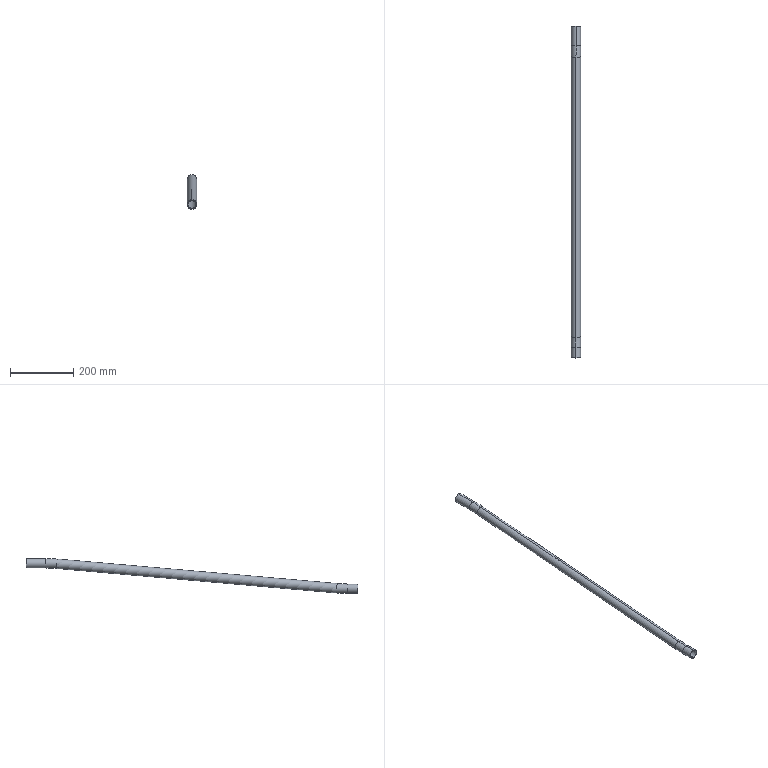Part | SolidWorks | features 3DProfileFeature 2, Sweep 1 | 1 solid | 22 faces | box 30 x 1053 x 110.793 mm | volume 185949 mm3 | cylinder 12 | torus 8 | plane 2 | commonest cylinder face diameters 26 x6 30 x6
STEP:
#1=CARTESIAN_POINT('',(19403.083,117.208,-3593.544));
#2=VERTEX_POINT('',#1);
#3=CARTESIAN_POINT('',(19403.083,114.942,-3567.643));
#4=VERTEX_POINT('',#3);
#5=CARTESIAN_POINT('',(19403.083,116.075,-3580.594));
#6=DIRECTION('',(0.,-0.9962,-0.08716));
#7=DIRECTION('',(0.,-0.08716,0.9962));
#8=AXIS2_PLACEMENT_3D('',#5,#6,#7);
#9=CIRCLE('',#8,13.);
#10=EDGE_CURVE('',#2,#4,#9,.T.);
#11=ORIENTED_EDGE('',*,*,#10,.T.);
#12=CARTESIAN_POINT('',(19403.083,150.937,-3566.072));
#13=VERTEX_POINT('',#12);
#14=CARTESIAN_POINT('',(19403.083,150.937,-3979.072));
#15=DIRECTION('',(-1.,0.,0.));
#16=DIRECTION('',(0.,-1.,0.));
#17=AXIS2_PLACEMENT_3D('',#14,#15,#16);
#18=CIRCLE('',#17,413.);
#19=EDGE_CURVE('',#4,#13,#18,.T.);
#20=ORIENTED_EDGE('',*,*,#19,.T.);
#21=CARTESIAN_POINT('',(19403.083,150.937,-3592.072));
#22=VERTEX_POINT('',#21);
#23=CARTESIAN_POINT('',(19403.083,150.937,-3579.072));
#24=DIRECTION('',(0.,-1.,0.));
#25=DIRECTION('',(0.,0.,-1.));
#26=AXIS2_PLACEMENT_3D('',#23,#24,#25);
#27=CIRCLE('',#26,13.);
#28=EDGE_CURVE('',#22,#13,#27,.T.);
#29=ORIENTED_EDGE('',*,*,#28,.F.);
#30=CARTESIAN_POINT('',(19403.083,150.937,-3979.072));
#31=DIRECTION('',(-1.,0.,0.));
#32=DIRECTION('',(0.,-1.,0.));
#33=AXIS2_PLACEMENT_3D('',#30,#31,#32);
#34=CIRCLE('',#33,387.);
#35=EDGE_CURVE('',#2,#22,#34,.T.);
#36=ORIENTED_EDGE('',*,*,#35,.F.);
#37=EDGE_LOOP('',(#11,#20,#29,#36));
#38=FACE_OUTER_BOUND('',#37,.T.);
#39=CARTESIAN_POINT('',(19403.083,150.937,-3979.072));
#40=DIRECTION('',(-1.,0.,0.));
#41=DIRECTION('',(0.,-1.,0.));
#42=AXIS2_PLACEMENT_3D('',#39,#40,#41);
#43=TOROIDAL_SURFACE('',#42,400.,13.);
#44=ADVANCED_FACE('',(#38),#43,.F.);
#45=CARTESIAN_POINT('',(19403.083,-807.464,-3646.865));
#46=VERTEX_POINT('',#45);
#47=CARTESIAN_POINT('',(19403.083,-807.464,-3672.865));
#48=VERTEX_POINT('',#47);
#49=CARTESIAN_POINT('',(19403.083,-807.464,-3659.865));
#50=DIRECTION('',(0.,-1.,0.));
#51=DIRECTION('',(0.,0.,1.));
#52=AXIS2_PLACEMENT_3D('',#49,#50,#51);
#53=CIRCLE('',#52,13.);
#54=EDGE_CURVE('',#46,#48,#53,.T.);
#55=ORIENTED_EDGE('',*,*,#54,.T.);
#56=CARTESIAN_POINT('',(19403.083,-771.469,-3671.293));
#57=VERTEX_POINT('',#56);
#58=CARTESIAN_POINT('',(19403.083,-807.464,-3259.865));
#59=DIRECTION('',(1.,0.,0.));
#60=DIRECTION('',(0.,0.,-1.));
#61=AXIS2_PLACEMENT_3D('',#58,#59,#60);
#62=CIRCLE('',#61,413.);
#63=EDGE_CURVE('',#48,#57,#62,.T.);
#64=ORIENTED_EDGE('',*,*,#63,.T.);
#65=CARTESIAN_POINT('',(19403.083,-773.735,-3645.392));
#66=VERTEX_POINT('',#65);
#67=CARTESIAN_POINT('',(19403.083,-772.602,-3658.343));
#68=DIRECTION('',(0.,-0.9962,-0.08716));
#69=DIRECTION('',(0.,0.08716,-0.9962));
#70=AXIS2_PLACEMENT_3D('',#67,#68,#69);
#71=CIRCLE('',#70,13.);
#72=EDGE_CURVE('',#66,#57,#71,.T.);
#73=ORIENTED_EDGE('',*,*,#72,.F.);
#74=CARTESIAN_POINT('',(19403.083,-807.464,-3259.865));
#75=DIRECTION('',(1.,0.,0.));
#76=DIRECTION('',(0.,0.,-1.));
#77=AXIS2_PLACEMENT_3D('',#74,#75,#76);
#78=CIRCLE('',#77,387.);
#79=EDGE_CURVE('',#46,#66,#78,.T.);
#80=ORIENTED_EDGE('',*,*,#79,.F.);
#81=EDGE_LOOP('',(#55,#64,#73,#80));
#82=FACE_OUTER_BOUND('',#81,.T.);
#83=CARTESIAN_POINT('',(19403.083,-807.464,-3259.865));
#84=DIRECTION('',(1.,0.,0.));
#85=DIRECTION('',(0.,0.,-1.));
#86=AXIS2_PLACEMENT_3D('',#83,#84,#85);
#87=TOROIDAL_SURFACE('',#86,400.,13.);
#88=ADVANCED_FACE('',(#82),#87,.F.);
#89=CARTESIAN_POINT('',(19403.083,114.767,-3565.651));
#90=VERTEX_POINT('',#89);
#91=CARTESIAN_POINT('',(19403.083,117.382,-3595.537));
#92=VERTEX_POINT('',#91);
#93=CARTESIAN_POINT('',(19403.083,116.075,-3580.594));
#94=DIRECTION('',(0.,-0.9962,-0.08716));
#95=DIRECTION('',(0.,0.08716,-0.9962));
#96=AXIS2_PLACEMENT_3D('',#93,#94,#95);
#97=CIRCLE('',#96,15.);
#98=EDGE_CURVE('',#90,#92,#97,.T.);
#99=ORIENTED_EDGE('',*,*,#98,.F.);
#100=CARTESIAN_POINT('',(19403.083,150.937,-3564.072));
#101=VERTEX_POINT('',#100);
#102=CARTESIAN_POINT('',(19403.083,150.937,-3979.072));
#103=DIRECTION('',(-1.,0.,0.));
#104=DIRECTION('',(0.,-1.,0.));
#105=AXIS2_PLACEMENT_3D('',#102,#103,#104);
#106=CIRCLE('',#105,415.);
#107=EDGE_CURVE('',#90,#101,#106,.T.);
#108=ORIENTED_EDGE('',*,*,#107,.T.);
#109=CARTESIAN_POINT('',(19403.083,150.937,-3594.072));
#110=VERTEX_POINT('',#109);
#111=CARTESIAN_POINT('',(19403.083,150.937,-3579.072));
#112=DIRECTION('',(0.,-1.,0.));
#113=DIRECTION('',(0.,0.,-1.));
#114=AXIS2_PLACEMENT_3D('',#111,#112,#113);
#115=CIRCLE('',#114,15.);
#116=EDGE_CURVE('',#101,#110,#115,.T.);
#117=ORIENTED_EDGE('',*,*,#116,.T.);
#118=CARTESIAN_POINT('',(19403.083,150.937,-3979.072));
#119=DIRECTION('',(-1.,0.,0.));
#120=DIRECTION('',(0.,-1.,0.));
#121=AXIS2_PLACEMENT_3D('',#118,#119,#120);
#122=CIRCLE('',#121,385.);
#123=EDGE_CURVE('',#92,#110,#122,.T.);
#124=ORIENTED_EDGE('',*,*,#123,.F.);
#125=EDGE_LOOP('',(#99,#108,#117,#124));
#126=FACE_OUTER_BOUND('',#125,.T.);
#127=CARTESIAN_POINT('',(19403.083,150.937,-3979.072));
#128=DIRECTION('',(-1.,0.,0.));
#129=DIRECTION('',(0.,-1.,0.));
#130=AXIS2_PLACEMENT_3D('',#127,#128,#129);
#131=TOROIDAL_SURFACE('',#130,400.,15.);
#132=ADVANCED_FACE('',(#126),#131,.T.);
#133=CARTESIAN_POINT('',(19403.083,-807.464,-3674.865));
#134=VERTEX_POINT('',#133);
#135=CARTESIAN_POINT('',(19403.083,-807.464,-3644.865));
#136=VERTEX_POINT('',#135);
#137=CARTESIAN_POINT('',(19403.083,-807.464,-3659.865));
#138=DIRECTION('',(0.,-1.,0.));
#139=DIRECTION('',(0.,0.,-1.));
#140=AXIS2_PLACEMENT_3D('',#137,#138,#139);
#141=CIRCLE('',#140,15.);
#142=EDGE_CURVE('',#134,#136,#141,.T.);
#143=ORIENTED_EDGE('',*,*,#142,.F.);
#144=CARTESIAN_POINT('',(19403.083,-771.295,-3673.286));
#145=VERTEX_POINT('',#144);
#146=CARTESIAN_POINT('',(19403.083,-807.464,-3259.865));
#147=DIRECTION('',(1.,0.,0.));
#148=DIRECTION('',(0.,0.,-1.));
#149=AXIS2_PLACEMENT_3D('',#146,#147,#148);
#150=CIRCLE('',#149,415.);
#151=EDGE_CURVE('',#134,#145,#150,.T.);
#152=ORIENTED_EDGE('',*,*,#151,.T.);
#153=CARTESIAN_POINT('',(19403.083,-773.909,-3643.4));
#154=VERTEX_POINT('',#153);
#155=CARTESIAN_POINT('',(19403.083,-772.602,-3658.343));
#156=DIRECTION('',(0.,-0.9962,-0.08716));
#157=DIRECTION('',(0.,0.08716,-0.9962));
#158=AXIS2_PLACEMENT_3D('',#155,#156,#157);
#159=CIRCLE('',#158,15.);
#160=EDGE_CURVE('',#145,#154,#159,.T.);
#161=ORIENTED_EDGE('',*,*,#160,.T.);
#162=CARTESIAN_POINT('',(19403.083,-807.464,-3259.865));
#163=DIRECTION('',(1.,0.,0.));
#164=DIRECTION('',(0.,0.,-1.));
#165=AXIS2_PLACEMENT_3D('',#162,#163,#164);
#166=CIRCLE('',#165,385.);
#167=EDGE_CURVE('',#136,#154,#166,.T.);
#168=ORIENTED_EDGE('',*,*,#167,.F.);
#169=EDGE_LOOP('',(#143,#152,#161,#168));
#170=FACE_OUTER_BOUND('',#169,.T.);
#171=CARTESIAN_POINT('',(19403.083,-807.464,-3259.865));
#172=DIRECTION('',(1.,0.,0.));
#173=DIRECTION('',(0.,0.,-1.));
#174=AXIS2_PLACEMENT_3D('',#171,#172,#173);
#175=TOROIDAL_SURFACE('',#174,400.,15.);
#176=ADVANCED_FACE('',(#170),#175,.T.);
#177=CARTESIAN_POINT('',(19403.083,150.937,-3579.072));
#178=DIRECTION('',(0.,-1.,0.));
#179=DIRECTION('',(0.,0.,-1.));
#180=AXIS2_PLACEMENT_3D('',#177,#178,#179);
#181=CIRCLE('',#180,13.);
#182=EDGE_CURVE('',#13,#22,#181,.T.);
#183=ORIENTED_EDGE('',*,*,#182,.T.);
#184=CARTESIAN_POINT('',(19403.083,213.472,-3592.072));
#185=VERTEX_POINT('',#184);
#186=CARTESIAN_POINT('',(19403.083,150.937,-3592.072));
#187=DIRECTION('',(0.,1.,0.));
#188=VECTOR('',#187,1000.);
#189=LINE('',#186,#188);
#190=EDGE_CURVE('',#22,#185,#189,.T.);
#191=ORIENTED_EDGE('',*,*,#190,.T.);
#192=CARTESIAN_POINT('',(19403.083,213.472,-3566.072));
#193=VERTEX_POINT('',#192);
#194=CARTESIAN_POINT('',(19403.083,213.472,-3579.072));
#195=DIRECTION('',(0.,-1.,0.));
#196=DIRECTION('',(0.,0.,-1.));
#197=AXIS2_PLACEMENT_3D('',#194,#195,#196);
#198=CIRCLE('',#197,13.);
#199=EDGE_CURVE('',#193,#185,#198,.T.);
#200=ORIENTED_EDGE('',*,*,#199,.F.);
#201=CARTESIAN_POINT('',(19403.083,150.937,-3566.072));
#202=DIRECTION('',(0.,1.,0.));
#203=VECTOR('',#202,1000.);
#204=LINE('',#201,#203);
#205=EDGE_CURVE('',#13,#193,#204,.T.);
#206=ORIENTED_EDGE('',*,*,#205,.F.);
#207=EDGE_LOOP('',(#183,#191,#200,#206));
#208=FACE_OUTER_BOUND('',#207,.T.);
#209=CARTESIAN_POINT('',(19403.083,150.937,-3579.072));
#210=DIRECTION('',(0.,1.,0.));
#211=DIRECTION('',(0.,0.,1.));
#212=AXIS2_PLACEMENT_3D('',#209,#210,#211);
#213=CYLINDRICAL_SURFACE('',#212,13.);
#214=ADVANCED_FACE('',(#208),#213,.F.);
#215=ORIENTED_EDGE('',*,*,#72,.T.);
#216=CARTESIAN_POINT('',(19403.083,-771.469,-3671.293));
#217=DIRECTION('',(0.,0.9962,0.08716));
#218=VECTOR('',#217,1000.);
#219=LINE('',#216,#218);
#220=EDGE_CURVE('',#57,#2,#219,.T.);
#221=ORIENTED_EDGE('',*,*,#220,.T.);
#222=CARTESIAN_POINT('',(19403.083,116.075,-3580.594));
#223=DIRECTION('',(0.,-0.9962,-0.08716));
#224=DIRECTION('',(0.,-0.08716,0.9962));
#225=AXIS2_PLACEMENT_3D('',#222,#223,#224);
#226=CIRCLE('',#225,13.);
#227=EDGE_CURVE('',#4,#2,#226,.T.);
#228=ORIENTED_EDGE('',*,*,#227,.F.);
#229=CARTESIAN_POINT('',(19403.083,-773.735,-3645.392));
#230=DIRECTION('',(0.,0.9962,0.08716));
#231=VECTOR('',#230,1000.);
#232=LINE('',#229,#231);
#233=EDGE_CURVE('',#66,#4,#232,.T.);
#234=ORIENTED_EDGE('',*,*,#233,.F.);
#235=EDGE_LOOP('',(#215,#221,#228,#234));
#236=FACE_OUTER_BOUND('',#235,.T.);
#237=CARTESIAN_POINT('',(19403.083,-772.602,-3658.343));
#238=DIRECTION('',(0.,0.9962,0.08716));
#239=DIRECTION('',(0.,-0.08716,0.9962));
#240=AXIS2_PLACEMENT_3D('',#237,#238,#239);
#241=CYLINDRICAL_SURFACE('',#240,13.);
#242=ADVANCED_FACE('',(#236),#241,.F.);
#243=CARTESIAN_POINT('',(19403.083,-840.,-3646.865));
#244=VERTEX_POINT('',#243);
#245=CARTESIAN_POINT('',(19403.083,-840.,-3672.865));
#246=VERTEX_POINT('',#245);
#247=CARTESIAN_POINT('',(19403.083,-840.,-3659.865));
#248=DIRECTION('',(0.,-1.,0.));
#249=DIRECTION('',(0.,0.,-1.));
#250=AXIS2_PLACEMENT_3D('',#247,#248,#249);
#251=CIRCLE('',#250,13.);
#252=EDGE_CURVE('',#244,#246,#251,.T.);
#253=ORIENTED_EDGE('',*,*,#252,.T.);
#254=CARTESIAN_POINT('',(19403.083,-840.,-3672.865));
#255=DIRECTION('',(0.,1.,0.));
#256=VECTOR('',#255,1000.);
#257=LINE('',#254,#256);
#258=EDGE_CURVE('',#246,#48,#257,.T.);
#259=ORIENTED_EDGE('',*,*,#258,.T.);
#260=ORIENTED_EDGE('',*,*,#54,.F.);
#261=CARTESIAN_POINT('',(19403.083,-840.,-3646.865));
#262=DIRECTION('',(0.,1.,0.));
#263=VECTOR('',#262,1000.);
#264=LINE('',#261,#263);
#265=EDGE_CURVE('',#244,#46,#264,.T.);
#266=ORIENTED_EDGE('',*,*,#265,.F.);
#267=EDGE_LOOP('',(#253,#259,#260,#266));
#268=FACE_OUTER_BOUND('',#267,.T.);
#269=CARTESIAN_POINT('',(19403.083,-840.,-3659.865));
#270=DIRECTION('',(0.,1.,0.));
#271=DIRECTION('',(0.,0.,1.));
#272=AXIS2_PLACEMENT_3D('',#269,#270,#271);
#273=CYLINDRICAL_SURFACE('',#272,13.);
#274=ADVANCED_FACE('',(#268),#273,.F.);
#275=CARTESIAN_POINT('',(19403.083,150.937,-3579.072));
#276=DIRECTION('',(0.,-1.,0.));
#277=DIRECTION('',(0.,0.,-1.));
#278=AXIS2_PLACEMENT_3D('',#275,#276,#277);
#279=CIRCLE('',#278,15.);
#280=EDGE_CURVE('',#110,#101,#279,.T.);
#281=ORIENTED_EDGE('',*,*,#280,.F.);
#282=CARTESIAN_POINT('',(19403.083,213.472,-3594.072));
#283=VERTEX_POINT('',#282);
#284=CARTESIAN_POINT('',(19403.083,150.937,-3594.072));
#285=DIRECTION('',(0.,1.,0.));
#286=VECTOR('',#285,1000.);
#287=LINE('',#284,#286);
#288=EDGE_CURVE('',#110,#283,#287,.T.);
#289=ORIENTED_EDGE('',*,*,#288,.T.);
#290=CARTESIAN_POINT('',(19403.083,213.472,-3564.072));
#291=VERTEX_POINT('',#290);
#292=CARTESIAN_POINT('',(19403.083,213.472,-3579.072));
#293=DIRECTION('',(0.,-1.,0.));
#294=DIRECTION('',(0.,0.,-1.));
#295=AXIS2_PLACEMENT_3D('',#292,#293,#294);
#296=CIRCLE('',#295,15.);
#297=EDGE_CURVE('',#283,#291,#296,.T.);
#298=ORIENTED_EDGE('',*,*,#297,.T.);
#299=CARTESIAN_POINT('',(19403.083,150.937,-3564.072));
#300=DIRECTION('',(0.,1.,0.));
#301=VECTOR('',#300,1000.);
#302=LINE('',#299,#301);
#303=EDGE_CURVE('',#101,#291,#302,.T.);
#304=ORIENTED_EDGE('',*,*,#303,.F.);
#305=EDGE_LOOP('',(#281,#289,#298,#304));
#306=FACE_OUTER_BOUND('',#305,.T.);
#307=CARTESIAN_POINT('',(19403.083,150.937,-3579.072));
#308=DIRECTION('',(0.,1.,0.));
#309=DIRECTION('',(0.,0.,1.));
#310=AXIS2_PLACEMENT_3D('',#307,#308,#309);
#311=CYLINDRICAL_SURFACE('',#310,15.);
#312=ADVANCED_FACE('',(#306),#311,.T.);
#313=ORIENTED_EDGE('',*,*,#160,.F.);
#314=CARTESIAN_POINT('',(19403.083,-771.295,-3673.286));
#315=DIRECTION('',(0.,0.9962,0.08716));
#316=VECTOR('',#315,1000.);
#317=LINE('',#314,#316);
#318=EDGE_CURVE('',#145,#92,#317,.T.);
#319=ORIENTED_EDGE('',*,*,#318,.T.);
#320=CARTESIAN_POINT('',(19403.083,116.075,-3580.594));
#321=DIRECTION('',(0.,-0.9962,-0.08716));
#322=DIRECTION('',(0.,0.08716,-0.9962));
#323=AXIS2_PLACEMENT_3D('',#320,#321,#322);
#324=CIRCLE('',#323,15.);
#325=EDGE_CURVE('',#92,#90,#324,.T.);
#326=ORIENTED_EDGE('',*,*,#325,.T.);
#327=CARTESIAN_POINT('',(19403.083,-773.909,-3643.4));
#328=DIRECTION('',(0.,0.9962,0.08716));
#329=VECTOR('',#328,1000.);
#330=LINE('',#327,#329);
#331=EDGE_CURVE('',#154,#90,#330,.T.);
#332=ORIENTED_EDGE('',*,*,#331,.F.);
#333=EDGE_LOOP('',(#313,#319,#326,#332));
#334=FACE_OUTER_BOUND('',#333,.T.);
#335=CARTESIAN_POINT('',(19403.083,-772.602,-3658.343));
#336=DIRECTION('',(0.,0.9962,0.08716));
#337=DIRECTION('',(0.,-0.08716,0.9962));
#338=AXIS2_PLACEMENT_3D('',#335,#336,#337);
#339=CYLINDRICAL_SURFACE('',#338,15.);
#340=ADVANCED_FACE('',(#334),#339,.T.);
#341=CARTESIAN_POINT('',(19403.083,-840.,-3674.865));
#342=VERTEX_POINT('',#341);
#343=CARTESIAN_POINT('',(19403.083,-840.,-3644.865));
#344=VERTEX_POINT('',#343);
#345=CARTESIAN_POINT('',(19403.083,-840.,-3659.865));
#346=DIRECTION('',(0.,-1.,0.));
#347=DIRECTION('',(0.,0.,-1.));
#348=AXIS2_PLACEMENT_3D('',#345,#346,#347);
#349=CIRCLE('',#348,15.);
#350=EDGE_CURVE('',#342,#344,#349,.T.);
#351=ORIENTED_EDGE('',*,*,#350,.F.);
#352=CARTESIAN_POINT('',(19403.083,-840.,-3674.865));
#353=DIRECTION('',(0.,1.,0.));
#354=VECTOR('',#353,1000.);
#355=LINE('',#352,#354);
#356=EDGE_CURVE('',#342,#134,#355,.T.);
#357=ORIENTED_EDGE('',*,*,#356,.T.);
#358=ORIENTED_EDGE('',*,*,#142,.T.);
#359=CARTESIAN_POINT('',(19403.083,-840.,-3644.865));
#360=DIRECTION('',(0.,1.,0.));
#361=VECTOR('',#360,1000.);
#362=LINE('',#359,#361);
#363=EDGE_CURVE('',#344,#136,#362,.T.);
#364=ORIENTED_EDGE('',*,*,#363,.F.);
#365=EDGE_LOOP('',(#351,#357,#358,#364));
#366=FACE_OUTER_BOUND('',#365,.T.);
#367=CARTESIAN_POINT('',(19403.083,-840.,-3659.865));
#368=DIRECTION('',(0.,1.,0.));
#369=DIRECTION('',(0.,0.,1.));
#370=AXIS2_PLACEMENT_3D('',#367,#368,#369);
#371=CYLINDRICAL_SURFACE('',#370,15.);
#372=ADVANCED_FACE('',(#366),#371,.T.);
#373=ORIENTED_EDGE('',*,*,#288,.F.);
#374=ORIENTED_EDGE('',*,*,#116,.F.);
#375=ORIENTED_EDGE('',*,*,#303,.T.);
#376=CARTESIAN_POINT('',(19403.083,213.472,-3579.072));
#377=DIRECTION('',(0.,-1.,0.));
#378=DIRECTION('',(0.,0.,-1.));
#379=AXIS2_PLACEMENT_3D('',#376,#377,#378);
#380=CIRCLE('',#379,15.);
#381=EDGE_CURVE('',#291,#283,#380,.T.);
#382=ORIENTED_EDGE('',*,*,#381,.T.);
#383=EDGE_LOOP('',(#373,#374,#375,#382));
#384=FACE_OUTER_BOUND('',#383,.T.);
#385=CARTESIAN_POINT('',(19403.083,150.937,-3579.072));
#386=DIRECTION('',(0.,1.,0.));
#387=DIRECTION('',(0.,0.,1.));
#388=AXIS2_PLACEMENT_3D('',#385,#386,#387);
#389=CYLINDRICAL_SURFACE('',#388,15.);
#390=ADVANCED_FACE('',(#384),#389,.T.);
#391=ORIENTED_EDGE('',*,*,#107,.F.);
#392=ORIENTED_EDGE('',*,*,#325,.F.);
#393=ORIENTED_EDGE('',*,*,#123,.T.);
#394=ORIENTED_EDGE('',*,*,#280,.T.);
#395=EDGE_LOOP('',(#391,#392,#393,#394));
#396=FACE_OUTER_BOUND('',#395,.T.);
#397=CARTESIAN_POINT('',(19403.083,150.937,-3979.072));
#398=DIRECTION('',(-1.,0.,0.));
#399=DIRECTION('',(0.,-1.,0.));
#400=AXIS2_PLACEMENT_3D('',#397,#398,#399);
#401=TOROIDAL_SURFACE('',#400,400.,15.);
#402=ADVANCED_FACE('',(#396),#401,.T.);
#403=ORIENTED_EDGE('',*,*,#318,.F.);
#404=CARTESIAN_POINT('',(19403.083,-772.602,-3658.343));
#405=DIRECTION('',(0.,-0.9962,-0.08716));
#406=DIRECTION('',(0.,0.08716,-0.9962));
#407=AXIS2_PLACEMENT_3D('',#404,#405,#406);
#408=CIRCLE('',#407,15.);
#409=EDGE_CURVE('',#154,#145,#408,.T.);
#410=ORIENTED_EDGE('',*,*,#409,.F.);
#411=ORIENTED_EDGE('',*,*,#331,.T.);
#412=ORIENTED_EDGE('',*,*,#98,.T.);
#413=EDGE_LOOP('',(#403,#410,#411,#412));
#414=FACE_OUTER_BOUND('',#413,.T.);
#415=CARTESIAN_POINT('',(19403.083,-772.602,-3658.343));
#416=DIRECTION('',(0.,0.9962,0.08716));
#417=DIRECTION('',(0.,-0.08716,0.9962));
#418=AXIS2_PLACEMENT_3D('',#415,#416,#417);
#419=CYLINDRICAL_SURFACE('',#418,15.);
#420=ADVANCED_FACE('',(#414),#419,.T.);
#421=ORIENTED_EDGE('',*,*,#151,.F.);
#422=CARTESIAN_POINT('',(19403.083,-807.464,-3659.865));
#423=DIRECTION('',(0.,-1.,0.));
#424=DIRECTION('',(0.,0.,-1.));
#425=AXIS2_PLACEMENT_3D('',#422,#423,#424);
#426=CIRCLE('',#425,15.);
#427=EDGE_CURVE('',#136,#134,#426,.T.);
#428=ORIENTED_EDGE('',*,*,#427,.F.);
#429=ORIENTED_EDGE('',*,*,#167,.T.);
#430=ORIENTED_EDGE('',*,*,#409,.T.);
#431=EDGE_LOOP('',(#421,#428,#429,#430));
#432=FACE_OUTER_BOUND('',#431,.T.);
#433=CARTESIAN_POINT('',(19403.083,-807.464,-3259.865));
#434=DIRECTION('',(1.,0.,0.));
#435=DIRECTION('',(0.,0.,-1.));
#436=AXIS2_PLACEMENT_3D('',#433,#434,#435);
#437=TOROIDAL_SURFACE('',#436,400.,15.);
#438=ADVANCED_FACE('',(#432),#437,.T.);
#439=ORIENTED_EDGE('',*,*,#356,.F.);
#440=CARTESIAN_POINT('',(19403.083,-840.,-3659.865));
#441=DIRECTION('',(0.,-1.,0.));
#442=DIRECTION('',(0.,0.,-1.));
#443=AXIS2_PLACEMENT_3D('',#440,#441,#442);
#444=CIRCLE('',#443,15.);
#445=EDGE_CURVE('',#344,#342,#444,.T.);
#446=ORIENTED_EDGE('',*,*,#445,.F.);
#447=ORIENTED_EDGE('',*,*,#363,.T.);
#448=ORIENTED_EDGE('',*,*,#427,.T.);
#449=EDGE_LOOP('',(#439,#446,#447,#448));
#450=FACE_OUTER_BOUND('',#449,.T.);
#451=CARTESIAN_POINT('',(19403.083,-840.,-3659.865));
#452=DIRECTION('',(0.,1.,0.));
#453=DIRECTION('',(0.,0.,1.));
#454=AXIS2_PLACEMENT_3D('',#451,#452,#453);
#455=CYLINDRICAL_SURFACE('',#454,15.);
#456=ADVANCED_FACE('',(#450),#455,.T.);
#457=ORIENTED_EDGE('',*,*,#199,.T.);
#458=CARTESIAN_POINT('',(19403.083,213.472,-3579.072));
#459=DIRECTION('',(0.,-1.,0.));
#460=DIRECTION('',(0.,0.,-1.));
#461=AXIS2_PLACEMENT_3D('',#458,#459,#460);
#462=CIRCLE('',#461,13.);
#463=EDGE_CURVE('',#185,#193,#462,.T.);
#464=ORIENTED_EDGE('',*,*,#463,.T.);
#465=EDGE_LOOP('',(#457,#464));
#466=FACE_BOUND('',#465,.T.);
#467=ORIENTED_EDGE('',*,*,#381,.F.);
#468=ORIENTED_EDGE('',*,*,#297,.F.);
#469=EDGE_LOOP('',(#467,#468));
#470=FACE_OUTER_BOUND('',#469,.T.);
#471=CARTESIAN_POINT('',(19403.083,213.472,-3579.072));
#472=DIRECTION('',(0.,-1.,0.));
#473=DIRECTION('',(0.,0.,-1.));
#474=AXIS2_PLACEMENT_3D('',#471,#472,#473);
#475=PLANE('',#474);
#476=ADVANCED_FACE('',(#466,#470),#475,.F.);
#477=ORIENTED_EDGE('',*,*,#252,.F.);
#478=CARTESIAN_POINT('',(19403.083,-840.,-3659.865));
#479=DIRECTION('',(0.,-1.,0.));
#480=DIRECTION('',(0.,0.,-1.));
#481=AXIS2_PLACEMENT_3D('',#478,#479,#480);
#482=CIRCLE('',#481,13.);
#483=EDGE_CURVE('',#246,#244,#482,.T.);
#484=ORIENTED_EDGE('',*,*,#483,.F.);
#485=EDGE_LOOP('',(#477,#484));
#486=FACE_BOUND('',#485,.T.);
#487=ORIENTED_EDGE('',*,*,#445,.T.);
#488=ORIENTED_EDGE('',*,*,#350,.T.);
#489=EDGE_LOOP('',(#487,#488));
#490=FACE_OUTER_BOUND('',#489,.T.);
#491=CARTESIAN_POINT('',(19403.083,-840.,-3659.865));
#492=DIRECTION('',(0.,-1.,0.));
#493=DIRECTION('',(0.,0.,-1.));
#494=AXIS2_PLACEMENT_3D('',#491,#492,#493);
#495=PLANE('',#494);
#496=ADVANCED_FACE('',(#486,#490),#495,.T.);
#497=ORIENTED_EDGE('',*,*,#190,.F.);
#498=ORIENTED_EDGE('',*,*,#28,.T.);
#499=ORIENTED_EDGE('',*,*,#205,.T.);
#500=ORIENTED_EDGE('',*,*,#463,.F.);
#501=EDGE_LOOP('',(#497,#498,#499,#500));
#502=FACE_OUTER_BOUND('',#501,.T.);
#503=CARTESIAN_POINT('',(19403.083,150.937,-3579.072));
#504=DIRECTION('',(0.,1.,0.));
#505=DIRECTION('',(0.,0.,1.));
#506=AXIS2_PLACEMENT_3D('',#503,#504,#505);
#507=CYLINDRICAL_SURFACE('',#506,13.);
#508=ADVANCED_FACE('',(#502),#507,.F.);
#509=ORIENTED_EDGE('',*,*,#19,.F.);
#510=ORIENTED_EDGE('',*,*,#227,.T.);
#511=ORIENTED_EDGE('',*,*,#35,.T.);
#512=ORIENTED_EDGE('',*,*,#182,.F.);
#513=EDGE_LOOP('',(#509,#510,#511,#512));
#514=FACE_OUTER_BOUND('',#513,.T.);
#515=CARTESIAN_POINT('',(19403.083,150.937,-3979.072));
#516=DIRECTION('',(-1.,0.,0.));
#517=DIRECTION('',(0.,-1.,0.));
#518=AXIS2_PLACEMENT_3D('',#515,#516,#517);
#519=TOROIDAL_SURFACE('',#518,400.,13.);
#520=ADVANCED_FACE('',(#514),#519,.F.);
#521=ORIENTED_EDGE('',*,*,#220,.F.);
#522=CARTESIAN_POINT('',(19403.083,-772.602,-3658.343));
#523=DIRECTION('',(0.,-0.9962,-0.08716));
#524=DIRECTION('',(0.,0.08716,-0.9962));
#525=AXIS2_PLACEMENT_3D('',#522,#523,#524);
#526=CIRCLE('',#525,13.);
#527=EDGE_CURVE('',#57,#66,#526,.T.);
#528=ORIENTED_EDGE('',*,*,#527,.T.);
#529=ORIENTED_EDGE('',*,*,#233,.T.);
#530=ORIENTED_EDGE('',*,*,#10,.F.);
#531=EDGE_LOOP('',(#521,#528,#529,#530));
#532=FACE_OUTER_BOUND('',#531,.T.);
#533=CARTESIAN_POINT('',(19403.083,-772.602,-3658.343));
#534=DIRECTION('',(0.,0.9962,0.08716));
#535=DIRECTION('',(0.,-0.08716,0.9962));
#536=AXIS2_PLACEMENT_3D('',#533,#534,#535);
#537=CYLINDRICAL_SURFACE('',#536,13.);
#538=ADVANCED_FACE('',(#532),#537,.F.);
#539=ORIENTED_EDGE('',*,*,#63,.F.);
#540=CARTESIAN_POINT('',(19403.083,-807.464,-3659.865));
#541=DIRECTION('',(0.,-1.,0.));
#542=DIRECTION('',(0.,0.,1.));
#543=AXIS2_PLACEMENT_3D('',#540,#541,#542);
#544=CIRCLE('',#543,13.);
#545=EDGE_CURVE('',#48,#46,#544,.T.);
#546=ORIENTED_EDGE('',*,*,#545,.T.);
#547=ORIENTED_EDGE('',*,*,#79,.T.);
#548=ORIENTED_EDGE('',*,*,#527,.F.);
#549=EDGE_LOOP('',(#539,#546,#547,#548));
#550=FACE_OUTER_BOUND('',#549,.T.);
#551=CARTESIAN_POINT('',(19403.083,-807.464,-3259.865));
#552=DIRECTION('',(1.,0.,0.));
#553=DIRECTION('',(0.,0.,-1.));
#554=AXIS2_PLACEMENT_3D('',#551,#552,#553);
#555=TOROIDAL_SURFACE('',#554,400.,13.);
#556=ADVANCED_FACE('',(#550),#555,.F.);
#557=ORIENTED_EDGE('',*,*,#258,.F.);
#558=ORIENTED_EDGE('',*,*,#483,.T.);
#559=ORIENTED_EDGE('',*,*,#265,.T.);
#560=ORIENTED_EDGE('',*,*,#545,.F.);
#561=EDGE_LOOP('',(#557,#558,#559,#560));
#562=FACE_OUTER_BOUND('',#561,.T.);
#563=CARTESIAN_POINT('',(19403.083,-840.,-3659.865));
#564=DIRECTION('',(0.,1.,0.));
#565=DIRECTION('',(0.,0.,1.));
#566=AXIS2_PLACEMENT_3D('',#563,#564,#565);
#567=CYLINDRICAL_SURFACE('',#566,13.);
#568=ADVANCED_FACE('',(#562),#567,.F.);
#569=CLOSED_SHELL('',(#44,#88,#132,#176,#214,#242,#274,#312,#340,#372,#390,#402,#420,#438,#456,#476,#496,#508,#520,#538,#556,#568));
#570=MANIFOLD_SOLID_BREP('',#569);
#571=CARTESIAN_POINT('',(0.,0.,0.));
#572=DIRECTION('',(0.,0.,1.));
#573=DIRECTION('',(1.,0.,0.));
#574=AXIS2_PLACEMENT_3D('',#571,#572,#573);
#575=(LENGTH_UNIT()NAMED_UNIT(*)SI_UNIT(.MILLI.,.METRE.));
#576=UNCERTAINTY_MEASURE_WITH_UNIT(LENGTH_MEASURE(0.00001),#575,'','');
#577=(NAMED_UNIT(*)PLANE_ANGLE_UNIT()SI_UNIT($,.RADIAN.));
#578=(NAMED_UNIT(*)SI_UNIT($,.STERADIAN.)SOLID_ANGLE_UNIT());
#579=(GEOMETRIC_REPRESENTATION_CONTEXT(3)GLOBAL_UNCERTAINTY_ASSIGNED_CONTEXT((#576))GLOBAL_UNIT_ASSIGNED_CONTEXT((#575,#577,#578))REPRESENTATION_CONTEXT('',''));
#580=ADVANCED_BREP_SHAPE_REPRESENTATION('',(#570,#574),#579);